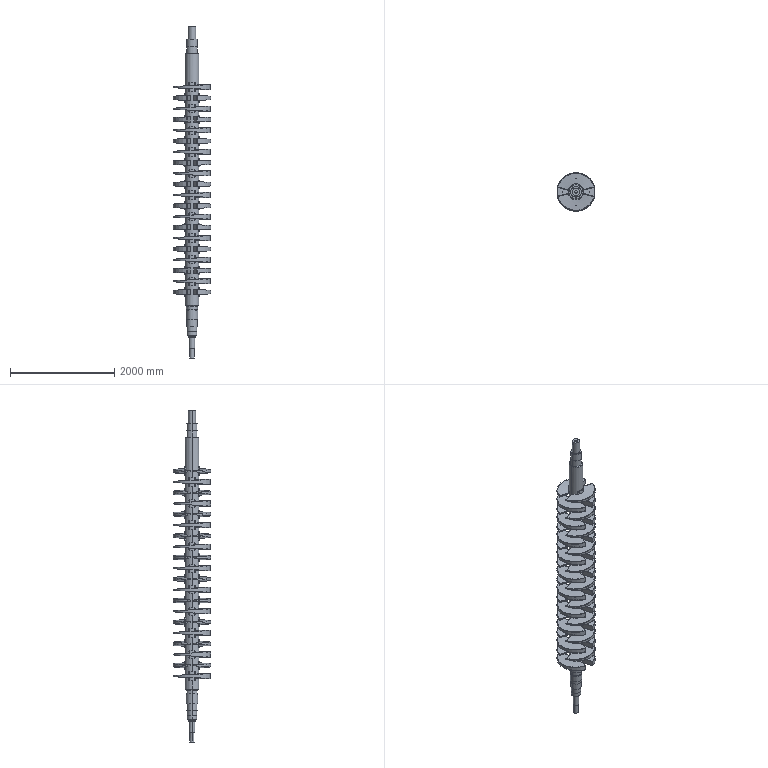Part | SolidWorks | features ReferencePattern 36, LocalLPattern 4, AEMSimFeature 1, RefAxis 1 | 330 solids | 3344 faces | volume 287612540 mm3 | cylinder 1314 | plane 1282 | spline 720 | cone 24 | torus 4 | commonest cylinder face diameters 18 x320 85 x164 20 x122 50 x82 15 x80 19 x80